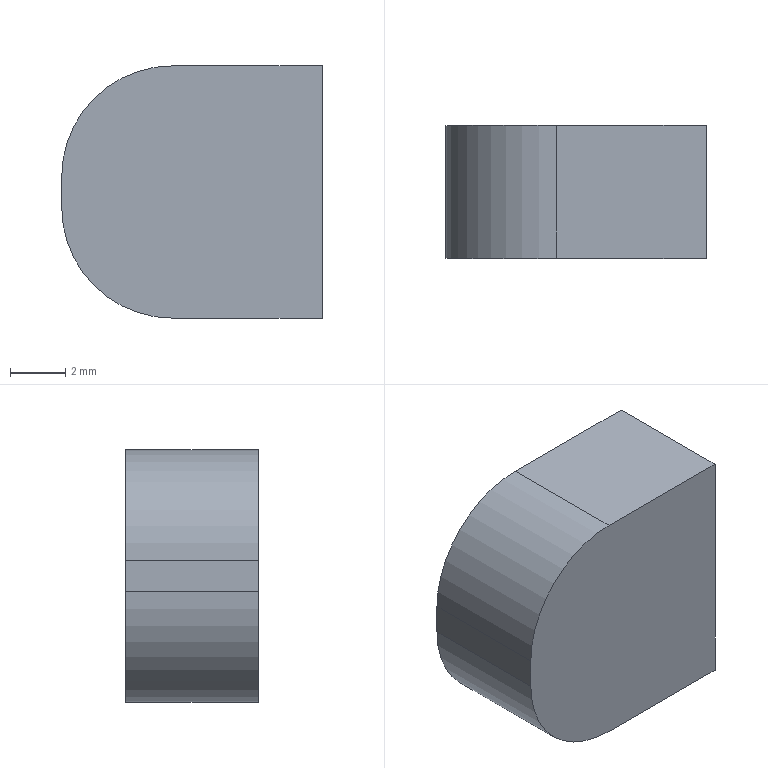Part | SolidWorks | features MBimport 1, Scale 1 | 1 solid | 17 faces | box 9.42 x 4.8 x 9.122 mm | volume 371.243 mm3 | plane 12 | cylinder 5 | commonest cylinder face diameters 1.578 x3 8 x2
STEP:
#1=CARTESIAN_POINT('',(-21.355,38.77,14.279));
#2=VERTEX_POINT('',#1);
#3=CARTESIAN_POINT('',(-21.355,38.37,14.279));
#4=VERTEX_POINT('',#3);
#5=CARTESIAN_POINT('',(-21.355,38.77,14.279));
#6=DIRECTION('',(0.,-1.,0.));
#7=VECTOR('',#6,1000.);
#8=LINE('',#5,#7);
#9=EDGE_CURVE('',#2,#4,#8,.T.);
#10=ORIENTED_EDGE('',*,*,#9,.F.);
#11=CARTESIAN_POINT('',(-22.144,38.77,15.069));
#12=VERTEX_POINT('',#11);
#13=CARTESIAN_POINT('',(-21.355,38.77,15.069));
#14=DIRECTION('',(0.,1.,0.));
#15=DIRECTION('',(0.,0.,1.));
#16=AXIS2_PLACEMENT_3D('',#13,#14,#15);
#17=CIRCLE('',#16,0.7892);
#18=EDGE_CURVE('',#2,#12,#17,.T.);
#19=ORIENTED_EDGE('',*,*,#18,.T.);
#20=CARTESIAN_POINT('',(-22.144,38.37,15.069));
#21=VERTEX_POINT('',#20);
#22=CARTESIAN_POINT('',(-22.144,38.77,15.069));
#23=DIRECTION('',(0.,-1.,0.));
#24=VECTOR('',#23,1000.);
#25=LINE('',#22,#24);
#26=EDGE_CURVE('',#12,#21,#25,.T.);
#27=ORIENTED_EDGE('',*,*,#26,.T.);
#28=CARTESIAN_POINT('',(-21.355,38.37,15.069));
#29=DIRECTION('',(0.,1.,0.));
#30=DIRECTION('',(0.,0.,1.));
#31=AXIS2_PLACEMENT_3D('',#28,#29,#30);
#32=CIRCLE('',#31,0.7892);
#33=EDGE_CURVE('',#4,#21,#32,.T.);
#34=ORIENTED_EDGE('',*,*,#33,.F.);
#35=EDGE_LOOP('',(#10,#19,#27,#34));
#36=FACE_OUTER_BOUND('',#35,.T.);
#37=CARTESIAN_POINT('',(-21.355,38.77,15.069));
#38=DIRECTION('',(0.,-1.,0.));
#39=DIRECTION('',(0.,0.,-1.));
#40=AXIS2_PLACEMENT_3D('',#37,#38,#39);
#41=CYLINDRICAL_SURFACE('',#40,0.7892);
#42=ADVANCED_FACE('',(#36),#41,.F.);
#43=CARTESIAN_POINT('',(-22.144,38.37,17.104));
#44=VERTEX_POINT('',#43);
#45=CARTESIAN_POINT('',(-20.566,38.37,17.104));
#46=VERTEX_POINT('',#45);
#47=CARTESIAN_POINT('',(-21.355,38.37,17.104));
#48=DIRECTION('',(0.,1.,0.));
#49=DIRECTION('',(0.,0.,1.));
#50=AXIS2_PLACEMENT_3D('',#47,#48,#49);
#51=CIRCLE('',#50,0.7892);
#52=EDGE_CURVE('',#44,#46,#51,.T.);
#53=ORIENTED_EDGE('',*,*,#52,.F.);
#54=CARTESIAN_POINT('',(-22.144,38.77,17.104));
#55=VERTEX_POINT('',#54);
#56=CARTESIAN_POINT('',(-22.144,38.77,17.104));
#57=DIRECTION('',(0.,-1.,0.));
#58=VECTOR('',#57,1000.);
#59=LINE('',#56,#58);
#60=EDGE_CURVE('',#55,#44,#59,.T.);
#61=ORIENTED_EDGE('',*,*,#60,.F.);
#62=CARTESIAN_POINT('',(-20.566,38.77,17.104));
#63=VERTEX_POINT('',#62);
#64=CARTESIAN_POINT('',(-21.355,38.77,17.104));
#65=DIRECTION('',(0.,1.,0.));
#66=DIRECTION('',(0.,0.,1.));
#67=AXIS2_PLACEMENT_3D('',#64,#65,#66);
#68=CIRCLE('',#67,0.7892);
#69=EDGE_CURVE('',#55,#63,#68,.T.);
#70=ORIENTED_EDGE('',*,*,#69,.T.);
#71=CARTESIAN_POINT('',(-20.566,38.77,17.104));
#72=DIRECTION('',(0.,-1.,0.));
#73=VECTOR('',#72,1000.);
#74=LINE('',#71,#73);
#75=EDGE_CURVE('',#63,#46,#74,.T.);
#76=ORIENTED_EDGE('',*,*,#75,.T.);
#77=EDGE_LOOP('',(#53,#61,#70,#76));
#78=FACE_OUTER_BOUND('',#77,.T.);
#79=CARTESIAN_POINT('',(-21.355,38.77,17.104));
#80=DIRECTION('',(0.,-1.,0.));
#81=DIRECTION('',(0.,0.,-1.));
#82=AXIS2_PLACEMENT_3D('',#79,#80,#81);
#83=CYLINDRICAL_SURFACE('',#82,0.7892);
#84=ADVANCED_FACE('',(#78),#83,.F.);
#85=CARTESIAN_POINT('',(-14.278,38.37,17.104));
#86=VERTEX_POINT('',#85);
#87=CARTESIAN_POINT('',(-14.278,38.37,15.069));
#88=VERTEX_POINT('',#87);
#89=CARTESIAN_POINT('',(-14.278,38.37,15.069));
#90=DIRECTION('',(0.,0.,-1.));
#91=VECTOR('',#90,1000.);
#92=LINE('',#89,#91);
#93=EDGE_CURVE('',#86,#88,#92,.T.);
#94=ORIENTED_EDGE('',*,*,#93,.T.);
#95=CARTESIAN_POINT('',(-20.566,38.37,15.069));
#96=VERTEX_POINT('',#95);
#97=CARTESIAN_POINT('',(-14.278,38.37,15.069));
#98=DIRECTION('',(-1.,0.,0.));
#99=VECTOR('',#98,1000.);
#100=LINE('',#97,#99);
#101=EDGE_CURVE('',#88,#96,#100,.T.);
#102=ORIENTED_EDGE('',*,*,#101,.T.);
#103=CARTESIAN_POINT('',(-21.355,38.37,15.069));
#104=DIRECTION('',(0.,1.,0.));
#105=DIRECTION('',(0.,0.,1.));
#106=AXIS2_PLACEMENT_3D('',#103,#104,#105);
#107=CIRCLE('',#106,0.7892);
#108=EDGE_CURVE('',#96,#4,#107,.T.);
#109=ORIENTED_EDGE('',*,*,#108,.T.);
#110=ORIENTED_EDGE('',*,*,#33,.T.);
#111=CARTESIAN_POINT('',(-23.466,38.37,15.069));
#112=VERTEX_POINT('',#111);
#113=CARTESIAN_POINT('',(-14.278,38.37,15.069));
#114=DIRECTION('',(-1.,0.,0.));
#115=VECTOR('',#114,1000.);
#116=LINE('',#113,#115);
#117=EDGE_CURVE('',#21,#112,#116,.T.);
#118=ORIENTED_EDGE('',*,*,#117,.T.);
#119=CARTESIAN_POINT('',(-23.466,38.37,17.104));
#120=VERTEX_POINT('',#119);
#121=CARTESIAN_POINT('',(-23.466,38.37,15.069));
#122=DIRECTION('',(0.,0.,1.));
#123=VECTOR('',#122,1000.);
#124=LINE('',#121,#123);
#125=EDGE_CURVE('',#112,#120,#124,.T.);
#126=ORIENTED_EDGE('',*,*,#125,.T.);
#127=CARTESIAN_POINT('',(-14.278,38.37,17.104));
#128=DIRECTION('',(1.,0.,0.));
#129=VECTOR('',#128,1000.);
#130=LINE('',#127,#129);
#131=EDGE_CURVE('',#120,#44,#130,.T.);
#132=ORIENTED_EDGE('',*,*,#131,.T.);
#133=ORIENTED_EDGE('',*,*,#52,.T.);
#134=CARTESIAN_POINT('',(-14.278,38.37,17.104));
#135=DIRECTION('',(1.,0.,0.));
#136=VECTOR('',#135,1000.);
#137=LINE('',#134,#136);
#138=EDGE_CURVE('',#46,#86,#137,.T.);
#139=ORIENTED_EDGE('',*,*,#138,.T.);
#140=EDGE_LOOP('',(#94,#102,#109,#110,#118,#126,#132,#133,#139));
#141=FACE_OUTER_BOUND('',#140,.T.);
#142=CARTESIAN_POINT('',(0.,38.37,0.));
#143=DIRECTION('',(0.,-1.,0.));
#144=DIRECTION('',(0.,0.,-1.));
#145=AXIS2_PLACEMENT_3D('',#142,#143,#144);
#146=PLANE('',#145);
#147=ADVANCED_FACE('',(#141),#146,.F.);
#148=CARTESIAN_POINT('',(-23.466,38.77,15.069));
#149=VERTEX_POINT('',#148);
#150=CARTESIAN_POINT('',(-23.466,38.77,17.104));
#151=VERTEX_POINT('',#150);
#152=CARTESIAN_POINT('',(-23.466,38.77,15.069));
#153=DIRECTION('',(0.,0.,1.));
#154=VECTOR('',#153,1000.);
#155=LINE('',#152,#154);
#156=EDGE_CURVE('',#149,#151,#155,.T.);
#157=ORIENTED_EDGE('',*,*,#156,.T.);
#158=CARTESIAN_POINT('',(-23.466,38.37,17.104));
#159=DIRECTION('',(0.,1.,0.));
#160=VECTOR('',#159,1000.);
#161=LINE('',#158,#160);
#162=EDGE_CURVE('',#120,#151,#161,.T.);
#163=ORIENTED_EDGE('',*,*,#162,.F.);
#164=ORIENTED_EDGE('',*,*,#125,.F.);
#165=CARTESIAN_POINT('',(-23.466,38.37,15.069));
#166=DIRECTION('',(0.,1.,0.));
#167=VECTOR('',#166,1000.);
#168=LINE('',#165,#167);
#169=EDGE_CURVE('',#112,#149,#168,.T.);
#170=ORIENTED_EDGE('',*,*,#169,.T.);
#171=EDGE_LOOP('',(#157,#163,#164,#170));
#172=FACE_OUTER_BOUND('',#171,.T.);
#173=CARTESIAN_POINT('',(-23.466,38.37,15.069));
#174=DIRECTION('',(-1.,0.,0.));
#175=DIRECTION('',(0.,0.,1.));
#176=AXIS2_PLACEMENT_3D('',#173,#174,#175);
#177=PLANE('',#176);
#178=ADVANCED_FACE('',(#172),#177,.F.);
#179=CARTESIAN_POINT('',(-23.698,38.77,16.695));
#180=VERTEX_POINT('',#179);
#181=CARTESIAN_POINT('',(-19.698,38.77,20.695));
#182=VERTEX_POINT('',#181);
#183=CARTESIAN_POINT('',(-19.698,38.77,16.695));
#184=DIRECTION('',(0.,1.,0.));
#185=DIRECTION('',(0.,0.,-1.));
#186=AXIS2_PLACEMENT_3D('',#183,#184,#185);
#187=CIRCLE('',#186,4.);
#188=EDGE_CURVE('',#180,#182,#187,.T.);
#189=ORIENTED_EDGE('',*,*,#188,.F.);
#190=CARTESIAN_POINT('',(-23.698,33.97,16.695));
#191=VERTEX_POINT('',#190);
#192=CARTESIAN_POINT('',(-23.698,38.77,16.695));
#193=DIRECTION('',(0.,1.,0.));
#194=VECTOR('',#193,1000.);
#195=LINE('',#192,#194);
#196=EDGE_CURVE('',#191,#180,#195,.T.);
#197=ORIENTED_EDGE('',*,*,#196,.F.);
#198=CARTESIAN_POINT('',(-19.698,33.97,20.695));
#199=VERTEX_POINT('',#198);
#200=CARTESIAN_POINT('',(-19.698,33.97,16.695));
#201=DIRECTION('',(0.,-1.,0.));
#202=DIRECTION('',(0.,0.,-1.));
#203=AXIS2_PLACEMENT_3D('',#200,#201,#202);
#204=CIRCLE('',#203,4.);
#205=EDGE_CURVE('',#199,#191,#204,.T.);
#206=ORIENTED_EDGE('',*,*,#205,.F.);
#207=CARTESIAN_POINT('',(-19.698,38.77,20.695));
#208=DIRECTION('',(0.,-1.,0.));
#209=VECTOR('',#208,1000.);
#210=LINE('',#207,#209);
#211=EDGE_CURVE('',#182,#199,#210,.T.);
#212=ORIENTED_EDGE('',*,*,#211,.F.);
#213=EDGE_LOOP('',(#189,#197,#206,#212));
#214=FACE_OUTER_BOUND('',#213,.T.);
#215=CARTESIAN_POINT('',(-19.698,38.77,16.695));
#216=DIRECTION('',(0.,-1.,0.));
#217=DIRECTION('',(0.,0.,-1.));
#218=AXIS2_PLACEMENT_3D('',#215,#216,#217);
#219=CYLINDRICAL_SURFACE('',#218,4.);
#220=ADVANCED_FACE('',(#214),#219,.T.);
#221=CARTESIAN_POINT('',(-19.698,38.77,11.573));
#222=VERTEX_POINT('',#221);
#223=CARTESIAN_POINT('',(-23.698,38.77,15.573));
#224=VERTEX_POINT('',#223);
#225=CARTESIAN_POINT('',(-19.698,38.77,15.573));
#226=DIRECTION('',(0.,1.,0.));
#227=DIRECTION('',(0.,0.,-1.));
#228=AXIS2_PLACEMENT_3D('',#225,#226,#227);
#229=CIRCLE('',#228,4.);
#230=EDGE_CURVE('',#222,#224,#229,.T.);
#231=ORIENTED_EDGE('',*,*,#230,.F.);
#232=CARTESIAN_POINT('',(-19.698,33.97,11.573));
#233=VERTEX_POINT('',#232);
#234=CARTESIAN_POINT('',(-19.698,38.77,11.573));
#235=DIRECTION('',(0.,1.,0.));
#236=VECTOR('',#235,1000.);
#237=LINE('',#234,#236);
#238=EDGE_CURVE('',#233,#222,#237,.T.);
#239=ORIENTED_EDGE('',*,*,#238,.F.);
#240=CARTESIAN_POINT('',(-23.698,33.97,15.573));
#241=VERTEX_POINT('',#240);
#242=CARTESIAN_POINT('',(-19.698,33.97,15.573));
#243=DIRECTION('',(0.,-1.,0.));
#244=DIRECTION('',(0.,0.,-1.));
#245=AXIS2_PLACEMENT_3D('',#242,#243,#244);
#246=CIRCLE('',#245,4.);
#247=EDGE_CURVE('',#241,#233,#246,.T.);
#248=ORIENTED_EDGE('',*,*,#247,.F.);
#249=CARTESIAN_POINT('',(-23.698,38.77,15.573));
#250=DIRECTION('',(0.,-1.,0.));
#251=VECTOR('',#250,1000.);
#252=LINE('',#249,#251);
#253=EDGE_CURVE('',#224,#241,#252,.T.);
#254=ORIENTED_EDGE('',*,*,#253,.F.);
#255=EDGE_LOOP('',(#231,#239,#248,#254));
#256=FACE_OUTER_BOUND('',#255,.T.);
#257=CARTESIAN_POINT('',(-19.698,38.77,15.573));
#258=DIRECTION('',(0.,-1.,0.));
#259=DIRECTION('',(0.,0.,-1.));
#260=AXIS2_PLACEMENT_3D('',#257,#258,#259);
#261=CYLINDRICAL_SURFACE('',#260,4.);
#262=ADVANCED_FACE('',(#256),#261,.T.);
#263=CARTESIAN_POINT('',(-23.698,33.97,11.573));
#264=DIRECTION('',(0.,0.,1.));
#265=VECTOR('',#264,1000.);
#266=LINE('',#263,#265);
#267=EDGE_CURVE('',#241,#191,#266,.T.);
#268=ORIENTED_EDGE('',*,*,#267,.F.);
#269=ORIENTED_EDGE('',*,*,#247,.T.);
#270=CARTESIAN_POINT('',(-14.278,33.97,11.573));
#271=VERTEX_POINT('',#270);
#272=CARTESIAN_POINT('',(-14.278,33.97,11.573));
#273=DIRECTION('',(-1.,0.,0.));
#274=VECTOR('',#273,1000.);
#275=LINE('',#272,#274);
#276=EDGE_CURVE('',#271,#233,#275,.T.);
#277=ORIENTED_EDGE('',*,*,#276,.F.);
#278=CARTESIAN_POINT('',(-14.278,33.97,20.695));
#279=VERTEX_POINT('',#278);
#280=CARTESIAN_POINT('',(-14.278,33.97,11.573));
#281=DIRECTION('',(0.,0.,-1.));
#282=VECTOR('',#281,1000.);
#283=LINE('',#280,#282);
#284=EDGE_CURVE('',#279,#271,#283,.T.);
#285=ORIENTED_EDGE('',*,*,#284,.F.);
#286=CARTESIAN_POINT('',(-14.278,33.97,20.695));
#287=DIRECTION('',(1.,0.,0.));
#288=VECTOR('',#287,1000.);
#289=LINE('',#286,#288);
#290=EDGE_CURVE('',#199,#279,#289,.T.);
#291=ORIENTED_EDGE('',*,*,#290,.F.);
#292=ORIENTED_EDGE('',*,*,#205,.T.);
#293=EDGE_LOOP('',(#268,#269,#277,#285,#291,#292));
#294=FACE_OUTER_BOUND('',#293,.T.);
#295=CARTESIAN_POINT('',(0.,33.97,0.));
#296=DIRECTION('',(0.,-1.,0.));
#297=DIRECTION('',(0.,0.,-1.));
#298=AXIS2_PLACEMENT_3D('',#295,#296,#297);
#299=PLANE('',#298);
#300=ADVANCED_FACE('',(#294),#299,.T.);
#301=CARTESIAN_POINT('',(-14.278,38.77,20.695));
#302=VERTEX_POINT('',#301);
#303=CARTESIAN_POINT('',(-14.278,38.77,20.695));
#304=DIRECTION('',(1.,0.,0.));
#305=VECTOR('',#304,1000.);
#306=LINE('',#303,#305);
#307=EDGE_CURVE('',#182,#302,#306,.T.);
#308=ORIENTED_EDGE('',*,*,#307,.F.);
#309=ORIENTED_EDGE('',*,*,#211,.T.);
#310=ORIENTED_EDGE('',*,*,#290,.T.);
#311=CARTESIAN_POINT('',(-14.278,38.77,20.695));
#312=DIRECTION('',(0.,-1.,0.));
#313=VECTOR('',#312,1000.);
#314=LINE('',#311,#313);
#315=EDGE_CURVE('',#302,#279,#314,.T.);
#316=ORIENTED_EDGE('',*,*,#315,.F.);
#317=EDGE_LOOP('',(#308,#309,#310,#316));
#318=FACE_OUTER_BOUND('',#317,.T.);
#319=CARTESIAN_POINT('',(-14.278,38.77,20.695));
#320=DIRECTION('',(0.,0.,-1.));
#321=DIRECTION('',(0.,-1.,0.));
#322=AXIS2_PLACEMENT_3D('',#319,#320,#321);
#323=PLANE('',#322);
#324=ADVANCED_FACE('',(#318),#323,.F.);
#325=CARTESIAN_POINT('',(-23.698,38.77,11.573));
#326=DIRECTION('',(0.,0.,1.));
#327=VECTOR('',#326,1000.);
#328=LINE('',#325,#327);
#329=EDGE_CURVE('',#224,#180,#328,.T.);
#330=ORIENTED_EDGE('',*,*,#329,.F.);
#331=ORIENTED_EDGE('',*,*,#253,.T.);
#332=ORIENTED_EDGE('',*,*,#267,.T.);
#333=ORIENTED_EDGE('',*,*,#196,.T.);
#334=EDGE_LOOP('',(#330,#331,#332,#333));
#335=FACE_OUTER_BOUND('',#334,.T.);
#336=CARTESIAN_POINT('',(-23.698,38.77,11.573));
#337=DIRECTION('',(1.,0.,0.));
#338=DIRECTION('',(0.,1.,0.));
#339=AXIS2_PLACEMENT_3D('',#336,#337,#338);
#340=PLANE('',#339);
#341=ADVANCED_FACE('',(#335),#340,.F.);
#342=ORIENTED_EDGE('',*,*,#276,.T.);
#343=ORIENTED_EDGE('',*,*,#238,.T.);
#344=CARTESIAN_POINT('',(-14.278,38.77,11.573));
#345=VERTEX_POINT('',#344);
#346=CARTESIAN_POINT('',(-14.278,38.77,11.573));
#347=DIRECTION('',(-1.,0.,0.));
#348=VECTOR('',#347,1000.);
#349=LINE('',#346,#348);
#350=EDGE_CURVE('',#345,#222,#349,.T.);
#351=ORIENTED_EDGE('',*,*,#350,.F.);
#352=CARTESIAN_POINT('',(-14.278,38.77,11.573));
#353=DIRECTION('',(0.,-1.,0.));
#354=VECTOR('',#353,1000.);
#355=LINE('',#352,#354);
#356=EDGE_CURVE('',#345,#271,#355,.T.);
#357=ORIENTED_EDGE('',*,*,#356,.T.);
#358=EDGE_LOOP('',(#342,#343,#351,#357));
#359=FACE_OUTER_BOUND('',#358,.T.);
#360=CARTESIAN_POINT('',(-14.278,38.77,11.573));
#361=DIRECTION('',(0.,0.,1.));
#362=DIRECTION('',(1.,0.,0.));
#363=AXIS2_PLACEMENT_3D('',#360,#361,#362);
#364=PLANE('',#363);
#365=ADVANCED_FACE('',(#359),#364,.F.);
#366=ORIENTED_EDGE('',*,*,#93,.F.);
#367=CARTESIAN_POINT('',(-14.278,38.77,17.104));
#368=VERTEX_POINT('',#367);
#369=CARTESIAN_POINT('',(-14.278,38.37,17.104));
#370=DIRECTION('',(0.,1.,0.));
#371=VECTOR('',#370,1000.);
#372=LINE('',#369,#371);
#373=EDGE_CURVE('',#86,#368,#372,.T.);
#374=ORIENTED_EDGE('',*,*,#373,.T.);
#375=CARTESIAN_POINT('',(-14.278,38.77,11.573));
#376=DIRECTION('',(0.,0.,-1.));
#377=VECTOR('',#376,1000.);
#378=LINE('',#375,#377);
#379=EDGE_CURVE('',#302,#368,#378,.T.);
#380=ORIENTED_EDGE('',*,*,#379,.F.);
#381=ORIENTED_EDGE('',*,*,#315,.T.);
#382=ORIENTED_EDGE('',*,*,#284,.T.);
#383=ORIENTED_EDGE('',*,*,#356,.F.);
#384=CARTESIAN_POINT('',(-14.278,38.77,15.069));
#385=VERTEX_POINT('',#384);
#386=CARTESIAN_POINT('',(-14.278,38.77,11.573));
#387=DIRECTION('',(0.,0.,-1.));
#388=VECTOR('',#387,1000.);
#389=LINE('',#386,#388);
#390=EDGE_CURVE('',#385,#345,#389,.T.);
#391=ORIENTED_EDGE('',*,*,#390,.F.);
#392=CARTESIAN_POINT('',(-14.278,38.37,15.069));
#393=DIRECTION('',(0.,1.,0.));
#394=VECTOR('',#393,1000.);
#395=LINE('',#392,#394);
#396=EDGE_CURVE('',#88,#385,#395,.T.);
#397=ORIENTED_EDGE('',*,*,#396,.F.);
#398=EDGE_LOOP('',(#366,#374,#380,#381,#382,#383,#391,#397));
#399=FACE_OUTER_BOUND('',#398,.T.);
#400=CARTESIAN_POINT('',(-14.278,38.77,11.573));
#401=DIRECTION('',(-1.,0.,0.));
#402=DIRECTION('',(0.,0.,1.));
#403=AXIS2_PLACEMENT_3D('',#400,#401,#402);
#404=PLANE('',#403);
#405=ADVANCED_FACE('',(#399),#404,.F.);
#406=ORIENTED_EDGE('',*,*,#26,.F.);
#407=CARTESIAN_POINT('',(-14.278,38.77,15.069));
#408=DIRECTION('',(-1.,0.,0.));
#409=VECTOR('',#408,1000.);
#410=LINE('',#407,#409);
#411=EDGE_CURVE('',#12,#149,#410,.T.);
#412=ORIENTED_EDGE('',*,*,#411,.T.);
#413=ORIENTED_EDGE('',*,*,#169,.F.);
#414=ORIENTED_EDGE('',*,*,#117,.F.);
#415=EDGE_LOOP('',(#406,#412,#413,#414));
#416=FACE_OUTER_BOUND('',#415,.T.);
#417=CARTESIAN_POINT('',(-14.278,38.37,15.069));
#418=DIRECTION('',(0.,0.,-1.));
#419=DIRECTION('',(0.,-1.,0.));
#420=AXIS2_PLACEMENT_3D('',#417,#418,#419);
#421=PLANE('',#420);
#422=ADVANCED_FACE('',(#416),#421,.F.);
#423=CARTESIAN_POINT('',(-20.566,38.77,15.069));
#424=VERTEX_POINT('',#423);
#425=CARTESIAN_POINT('',(-20.566,38.77,15.069));
#426=DIRECTION('',(0.,-1.,0.));
#427=VECTOR('',#426,1000.);
#428=LINE('',#425,#427);
#429=EDGE_CURVE('',#424,#96,#428,.T.);
#430=ORIENTED_EDGE('',*,*,#429,.T.);
#431=ORIENTED_EDGE('',*,*,#101,.F.);
#432=ORIENTED_EDGE('',*,*,#396,.T.);
#433=CARTESIAN_POINT('',(-14.278,38.77,15.069));
#434=DIRECTION('',(-1.,0.,0.));
#435=VECTOR('',#434,1000.);
#436=LINE('',#433,#435);
#437=EDGE_CURVE('',#385,#424,#436,.T.);
#438=ORIENTED_EDGE('',*,*,#437,.T.);
#439=EDGE_LOOP('',(#430,#431,#432,#438));
#440=FACE_OUTER_BOUND('',#439,.T.);
#441=CARTESIAN_POINT('',(-14.278,38.37,15.069));
#442=DIRECTION('',(0.,0.,-1.));
#443=DIRECTION('',(0.,-1.,0.));
#444=AXIS2_PLACEMENT_3D('',#441,#442,#443);
#445=PLANE('',#444);
#446=ADVANCED_FACE('',(#440),#445,.F.);
#447=ORIENTED_EDGE('',*,*,#75,.F.);
#448=CARTESIAN_POINT('',(-14.278,38.77,17.104));
#449=DIRECTION('',(1.,0.,0.));
#450=VECTOR('',#449,1000.);
#451=LINE('',#448,#450);
#452=EDGE_CURVE('',#63,#368,#451,.T.);
#453=ORIENTED_EDGE('',*,*,#452,.T.);
#454=ORIENTED_EDGE('',*,*,#373,.F.);
#455=ORIENTED_EDGE('',*,*,#138,.F.);
#456=EDGE_LOOP('',(#447,#453,#454,#455));
#457=FACE_OUTER_BOUND('',#456,.T.);
#458=CARTESIAN_POINT('',(-14.278,38.37,17.104));
#459=DIRECTION('',(0.,0.,1.));
#460=DIRECTION('',(1.,0.,0.));
#461=AXIS2_PLACEMENT_3D('',#458,#459,#460);
#462=PLANE('',#461);
#463=ADVANCED_FACE('',(#457),#462,.F.);
#464=ORIENTED_EDGE('',*,*,#60,.T.);
#465=ORIENTED_EDGE('',*,*,#131,.F.);
#466=ORIENTED_EDGE('',*,*,#162,.T.);
#467=CARTESIAN_POINT('',(-14.278,38.77,17.104));
#468=DIRECTION('',(1.,0.,0.));
#469=VECTOR('',#468,1000.);
#470=LINE('',#467,#469);
#471=EDGE_CURVE('',#151,#55,#470,.T.);
#472=ORIENTED_EDGE('',*,*,#471,.T.);
#473=EDGE_LOOP('',(#464,#465,#466,#472));
#474=FACE_OUTER_BOUND('',#473,.T.);
#475=CARTESIAN_POINT('',(-14.278,38.37,17.104));
#476=DIRECTION('',(0.,0.,1.));
#477=DIRECTION('',(1.,0.,0.));
#478=AXIS2_PLACEMENT_3D('',#475,#476,#477);
#479=PLANE('',#478);
#480=ADVANCED_FACE('',(#474),#479,.F.);
#481=CARTESIAN_POINT('',(-21.355,38.77,15.069));
#482=DIRECTION('',(0.,1.,0.));
#483=DIRECTION('',(0.,0.,1.));
#484=AXIS2_PLACEMENT_3D('',#481,#482,#483);
#485=CIRCLE('',#484,0.7892);
#486=EDGE_CURVE('',#424,#2,#485,.T.);
#487=ORIENTED_EDGE('',*,*,#486,.F.);
#488=ORIENTED_EDGE('',*,*,#437,.F.);
#489=ORIENTED_EDGE('',*,*,#390,.T.);
#490=ORIENTED_EDGE('',*,*,#350,.T.);
#491=ORIENTED_EDGE('',*,*,#230,.T.);
#492=ORIENTED_EDGE('',*,*,#329,.T.);
#493=ORIENTED_EDGE('',*,*,#188,.T.);
#494=ORIENTED_EDGE('',*,*,#307,.T.);
#495=ORIENTED_EDGE('',*,*,#379,.T.);
#496=ORIENTED_EDGE('',*,*,#452,.F.);
#497=ORIENTED_EDGE('',*,*,#69,.F.);
#498=ORIENTED_EDGE('',*,*,#471,.F.);
#499=ORIENTED_EDGE('',*,*,#156,.F.);
#500=ORIENTED_EDGE('',*,*,#411,.F.);
#501=ORIENTED_EDGE('',*,*,#18,.F.);
#502=EDGE_LOOP('',(#487,#488,#489,#490,#491,#492,#493,#494,#495,#496,#497,#498,#499,#500,#501));
#503=FACE_OUTER_BOUND('',#502,.T.);
#504=CARTESIAN_POINT('',(0.,38.77,0.));
#505=DIRECTION('',(0.,-1.,0.));
#506=DIRECTION('',(0.,0.,-1.));
#507=AXIS2_PLACEMENT_3D('',#504,#505,#506);
#508=PLANE('',#507);
#509=ADVANCED_FACE('',(#503),#508,.F.);
#510=ORIENTED_EDGE('',*,*,#486,.T.);
#511=ORIENTED_EDGE('',*,*,#9,.T.);
#512=ORIENTED_EDGE('',*,*,#108,.F.);
#513=ORIENTED_EDGE('',*,*,#429,.F.);
#514=EDGE_LOOP('',(#510,#511,#512,#513));
#515=FACE_OUTER_BOUND('',#514,.T.);
#516=CARTESIAN_POINT('',(-21.355,38.77,15.069));
#517=DIRECTION('',(0.,-1.,0.));
#518=DIRECTION('',(0.,0.,-1.));
#519=AXIS2_PLACEMENT_3D('',#516,#517,#518);
#520=CYLINDRICAL_SURFACE('',#519,0.7892);
#521=ADVANCED_FACE('',(#515),#520,.F.);
#522=CLOSED_SHELL('',(#42,#84,#147,#178,#220,#262,#300,#324,#341,#365,#405,#422,#446,#463,#480,#509,#521));
#523=MANIFOLD_SOLID_BREP('',#522);
#524=CARTESIAN_POINT('',(0.,0.,0.));
#525=DIRECTION('',(0.,0.,1.));
#526=DIRECTION('',(1.,0.,0.));
#527=AXIS2_PLACEMENT_3D('',#524,#525,#526);
#528=(LENGTH_UNIT()NAMED_UNIT(*)SI_UNIT(.MILLI.,.METRE.));
#529=UNCERTAINTY_MEASURE_WITH_UNIT(LENGTH_MEASURE(0.00001),#528,'','');
#530=(NAMED_UNIT(*)PLANE_ANGLE_UNIT()SI_UNIT($,.RADIAN.));
#531=(NAMED_UNIT(*)SI_UNIT($,.STERADIAN.)SOLID_ANGLE_UNIT());
#532=(GEOMETRIC_REPRESENTATION_CONTEXT(3)GLOBAL_UNCERTAINTY_ASSIGNED_CONTEXT((#529))GLOBAL_UNIT_ASSIGNED_CONTEXT((#528,#530,#531))REPRESENTATION_CONTEXT('',''));
#533=ADVANCED_BREP_SHAPE_REPRESENTATION('',(#523,#527),#532);